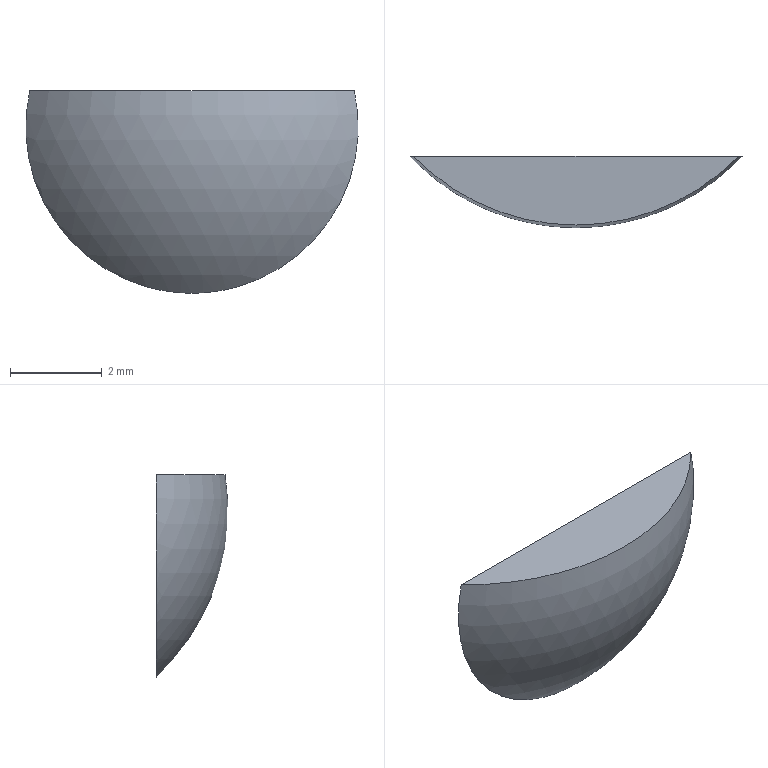Part | STEP file | solid 217 | 1 solid | 3 faces | box 7.264 x 1.563 x 4.422 mm | volume 23.265 mm3 | plane 2 | sphere 1